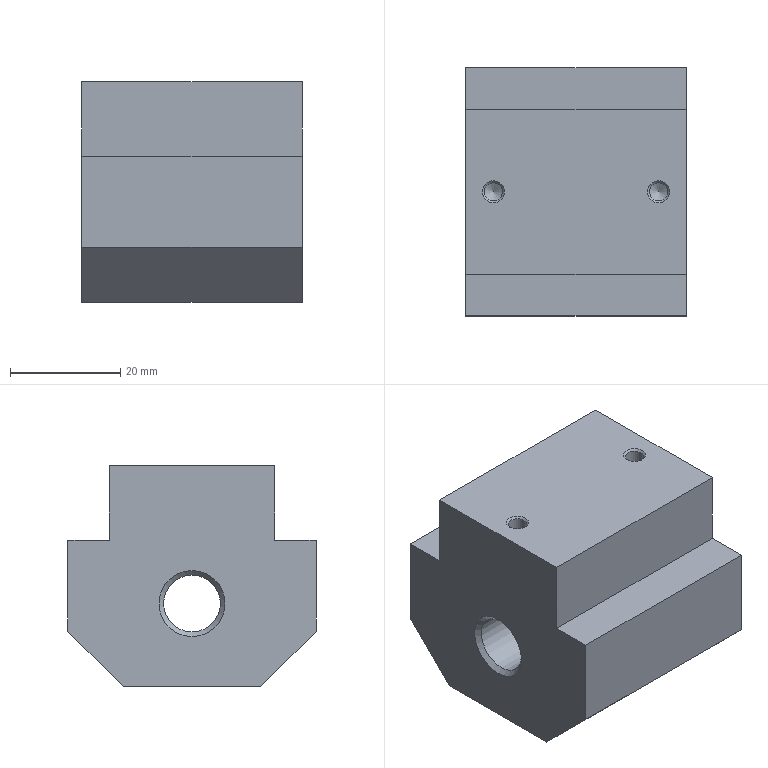Part | STEP file | Tube feed_id786_x_t | 1 solid | 25 faces | box 40 x 45 x 40 mm | volume 56393 mm3 | plane 14 | cone 8 | cylinder 3 | commonest cylinder face diameters 3.3 x2 10.3 x1